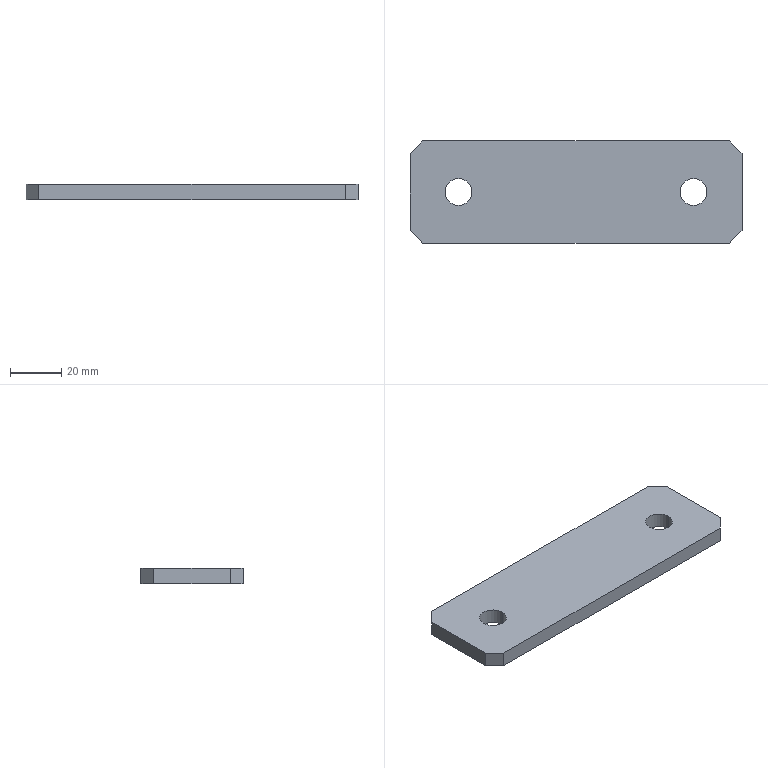Part | SolidWorks | features Extrusion 1 | 1 solid | 14 faces | box 130 x 40 x 6 mm | volume 29861 mm3 | plane 10 | cylinder 4 | commonest cylinder face diameters 10.5 x4
STEP:
#1=CARTESIAN_POINT('',(40.75,0.,3.));
#2=VERTEX_POINT('',#1);
#3=CARTESIAN_POINT('',(51.25,0.,3.));
#4=VERTEX_POINT('',#3);
#5=CARTESIAN_POINT('',(46.,0.,3.));
#6=DIRECTION('',(0.,0.,1.));
#7=DIRECTION('',(1.,0.,0.));
#8=AXIS2_PLACEMENT_3D('',#5,#6,#7);
#9=CIRCLE('',#8,5.25);
#10=EDGE_CURVE('',#2,#4,#9,.T.);
#11=ORIENTED_EDGE('',*,*,#10,.T.);
#12=CARTESIAN_POINT('',(51.25,0.,-3.));
#13=VERTEX_POINT('',#12);
#14=CARTESIAN_POINT('',(51.25,0.,3.));
#15=DIRECTION('',(0.,0.,-1.));
#16=VECTOR('',#15,1000.);
#17=LINE('',#14,#16);
#18=EDGE_CURVE('',#4,#13,#17,.T.);
#19=ORIENTED_EDGE('',*,*,#18,.T.);
#20=CARTESIAN_POINT('',(40.75,0.,-3.));
#21=VERTEX_POINT('',#20);
#22=CARTESIAN_POINT('',(46.,0.,-3.));
#23=DIRECTION('',(0.,0.,1.));
#24=DIRECTION('',(1.,0.,0.));
#25=AXIS2_PLACEMENT_3D('',#22,#23,#24);
#26=CIRCLE('',#25,5.25);
#27=EDGE_CURVE('',#21,#13,#26,.T.);
#28=ORIENTED_EDGE('',*,*,#27,.F.);
#29=CARTESIAN_POINT('',(40.75,0.,3.));
#30=DIRECTION('',(0.,0.,-1.));
#31=VECTOR('',#30,1000.);
#32=LINE('',#29,#31);
#33=EDGE_CURVE('',#2,#21,#32,.T.);
#34=ORIENTED_EDGE('',*,*,#33,.F.);
#35=EDGE_LOOP('',(#11,#19,#28,#34));
#36=FACE_OUTER_BOUND('',#35,.T.);
#37=CARTESIAN_POINT('',(46.,0.,3.));
#38=DIRECTION('',(0.,0.,-1.));
#39=DIRECTION('',(-1.,0.,0.));
#40=AXIS2_PLACEMENT_3D('',#37,#38,#39);
#41=CYLINDRICAL_SURFACE('',#40,5.25);
#42=ADVANCED_FACE('',(#36),#41,.F.);
#43=CARTESIAN_POINT('',(-51.25,0.,3.));
#44=VERTEX_POINT('',#43);
#45=CARTESIAN_POINT('',(-40.75,0.,3.));
#46=VERTEX_POINT('',#45);
#47=CARTESIAN_POINT('',(-46.,0.,3.));
#48=DIRECTION('',(0.,0.,1.));
#49=DIRECTION('',(1.,0.,0.));
#50=AXIS2_PLACEMENT_3D('',#47,#48,#49);
#51=CIRCLE('',#50,5.25);
#52=EDGE_CURVE('',#44,#46,#51,.T.);
#53=ORIENTED_EDGE('',*,*,#52,.T.);
#54=CARTESIAN_POINT('',(-40.75,0.,-3.));
#55=VERTEX_POINT('',#54);
#56=CARTESIAN_POINT('',(-40.75,0.,3.));
#57=DIRECTION('',(0.,0.,-1.));
#58=VECTOR('',#57,1000.);
#59=LINE('',#56,#58);
#60=EDGE_CURVE('',#46,#55,#59,.T.);
#61=ORIENTED_EDGE('',*,*,#60,.T.);
#62=CARTESIAN_POINT('',(-51.25,0.,-3.));
#63=VERTEX_POINT('',#62);
#64=CARTESIAN_POINT('',(-46.,0.,-3.));
#65=DIRECTION('',(0.,0.,1.));
#66=DIRECTION('',(1.,0.,0.));
#67=AXIS2_PLACEMENT_3D('',#64,#65,#66);
#68=CIRCLE('',#67,5.25);
#69=EDGE_CURVE('',#63,#55,#68,.T.);
#70=ORIENTED_EDGE('',*,*,#69,.F.);
#71=CARTESIAN_POINT('',(-51.25,0.,3.));
#72=DIRECTION('',(0.,0.,-1.));
#73=VECTOR('',#72,1000.);
#74=LINE('',#71,#73);
#75=EDGE_CURVE('',#44,#63,#74,.T.);
#76=ORIENTED_EDGE('',*,*,#75,.F.);
#77=EDGE_LOOP('',(#53,#61,#70,#76));
#78=FACE_OUTER_BOUND('',#77,.T.);
#79=CARTESIAN_POINT('',(-46.,0.,3.));
#80=DIRECTION('',(0.,0.,-1.));
#81=DIRECTION('',(-1.,0.,0.));
#82=AXIS2_PLACEMENT_3D('',#79,#80,#81);
#83=CYLINDRICAL_SURFACE('',#82,5.25);
#84=ADVANCED_FACE('',(#78),#83,.F.);
#85=ORIENTED_EDGE('',*,*,#52,.F.);
#86=CARTESIAN_POINT('',(-46.,0.,3.));
#87=DIRECTION('',(0.,0.,1.));
#88=DIRECTION('',(1.,0.,0.));
#89=AXIS2_PLACEMENT_3D('',#86,#87,#88);
#90=CIRCLE('',#89,5.25);
#91=EDGE_CURVE('',#46,#44,#90,.T.);
#92=ORIENTED_EDGE('',*,*,#91,.F.);
#93=EDGE_LOOP('',(#85,#92));
#94=FACE_BOUND('',#93,.T.);
#95=CARTESIAN_POINT('',(-65.,15.,3.));
#96=VERTEX_POINT('',#95);
#97=CARTESIAN_POINT('',(-65.,-15.,3.));
#98=VERTEX_POINT('',#97);
#99=CARTESIAN_POINT('',(-65.,-15.,3.));
#100=DIRECTION('',(0.,-1.,0.));
#101=VECTOR('',#100,1000.);
#102=LINE('',#99,#101);
#103=EDGE_CURVE('',#96,#98,#102,.T.);
#104=ORIENTED_EDGE('',*,*,#103,.T.);
#105=CARTESIAN_POINT('',(-60.,-20.,3.));
#106=VERTEX_POINT('',#105);
#107=CARTESIAN_POINT('',(-60.,-20.,3.));
#108=DIRECTION('',(0.7071,-0.7071,0.));
#109=VECTOR('',#108,1000.);
#110=LINE('',#107,#109);
#111=EDGE_CURVE('',#98,#106,#110,.T.);
#112=ORIENTED_EDGE('',*,*,#111,.T.);
#113=CARTESIAN_POINT('',(60.,-20.,3.));
#114=VERTEX_POINT('',#113);
#115=CARTESIAN_POINT('',(60.,-20.,3.));
#116=DIRECTION('',(1.,0.,0.));
#117=VECTOR('',#116,1000.);
#118=LINE('',#115,#117);
#119=EDGE_CURVE('',#106,#114,#118,.T.);
#120=ORIENTED_EDGE('',*,*,#119,.T.);
#121=CARTESIAN_POINT('',(65.,-15.,3.));
#122=VERTEX_POINT('',#121);
#123=CARTESIAN_POINT('',(65.,-15.,3.));
#124=DIRECTION('',(0.7071,0.7071,0.));
#125=VECTOR('',#124,1000.);
#126=LINE('',#123,#125);
#127=EDGE_CURVE('',#114,#122,#126,.T.);
#128=ORIENTED_EDGE('',*,*,#127,.T.);
#129=CARTESIAN_POINT('',(65.,15.,3.));
#130=VERTEX_POINT('',#129);
#131=CARTESIAN_POINT('',(65.,-15.,3.));
#132=DIRECTION('',(0.,1.,0.));
#133=VECTOR('',#132,1000.);
#134=LINE('',#131,#133);
#135=EDGE_CURVE('',#122,#130,#134,.T.);
#136=ORIENTED_EDGE('',*,*,#135,.T.);
#137=CARTESIAN_POINT('',(60.,20.,3.));
#138=VERTEX_POINT('',#137);
#139=CARTESIAN_POINT('',(65.,15.,3.));
#140=DIRECTION('',(-0.7071,0.7071,0.));
#141=VECTOR('',#140,1000.);
#142=LINE('',#139,#141);
#143=EDGE_CURVE('',#130,#138,#142,.T.);
#144=ORIENTED_EDGE('',*,*,#143,.T.);
#145=CARTESIAN_POINT('',(-60.,20.,3.));
#146=VERTEX_POINT('',#145);
#147=CARTESIAN_POINT('',(60.,20.,3.));
#148=DIRECTION('',(-1.,0.,0.));
#149=VECTOR('',#148,1000.);
#150=LINE('',#147,#149);
#151=EDGE_CURVE('',#138,#146,#150,.T.);
#152=ORIENTED_EDGE('',*,*,#151,.T.);
#153=CARTESIAN_POINT('',(-65.,15.,3.));
#154=DIRECTION('',(-0.7071,-0.7071,0.));
#155=VECTOR('',#154,1000.);
#156=LINE('',#153,#155);
#157=EDGE_CURVE('',#146,#96,#156,.T.);
#158=ORIENTED_EDGE('',*,*,#157,.T.);
#159=EDGE_LOOP('',(#104,#112,#120,#128,#136,#144,#152,#158));
#160=FACE_OUTER_BOUND('',#159,.T.);
#161=ORIENTED_EDGE('',*,*,#10,.F.);
#162=CARTESIAN_POINT('',(46.,0.,3.));
#163=DIRECTION('',(0.,0.,1.));
#164=DIRECTION('',(1.,0.,0.));
#165=AXIS2_PLACEMENT_3D('',#162,#163,#164);
#166=CIRCLE('',#165,5.25);
#167=EDGE_CURVE('',#4,#2,#166,.T.);
#168=ORIENTED_EDGE('',*,*,#167,.F.);
#169=EDGE_LOOP('',(#161,#168));
#170=FACE_BOUND('',#169,.T.);
#171=CARTESIAN_POINT('',(0.,0.,3.));
#172=DIRECTION('',(0.,0.,1.));
#173=DIRECTION('',(1.,0.,0.));
#174=AXIS2_PLACEMENT_3D('',#171,#172,#173);
#175=PLANE('',#174);
#176=ADVANCED_FACE('',(#94,#160,#170),#175,.T.);
#177=CARTESIAN_POINT('',(-65.,15.,-3.));
#178=VERTEX_POINT('',#177);
#179=CARTESIAN_POINT('',(-65.,-15.,-3.));
#180=VERTEX_POINT('',#179);
#181=CARTESIAN_POINT('',(-65.,-15.,-3.));
#182=DIRECTION('',(0.,-1.,0.));
#183=VECTOR('',#182,1000.);
#184=LINE('',#181,#183);
#185=EDGE_CURVE('',#178,#180,#184,.T.);
#186=ORIENTED_EDGE('',*,*,#185,.F.);
#187=CARTESIAN_POINT('',(-60.,20.,-3.));
#188=VERTEX_POINT('',#187);
#189=CARTESIAN_POINT('',(-65.,15.,-3.));
#190=DIRECTION('',(-0.7071,-0.7071,0.));
#191=VECTOR('',#190,1000.);
#192=LINE('',#189,#191);
#193=EDGE_CURVE('',#188,#178,#192,.T.);
#194=ORIENTED_EDGE('',*,*,#193,.F.);
#195=CARTESIAN_POINT('',(60.,20.,-3.));
#196=VERTEX_POINT('',#195);
#197=CARTESIAN_POINT('',(60.,20.,-3.));
#198=DIRECTION('',(-1.,0.,0.));
#199=VECTOR('',#198,1000.);
#200=LINE('',#197,#199);
#201=EDGE_CURVE('',#196,#188,#200,.T.);
#202=ORIENTED_EDGE('',*,*,#201,.F.);
#203=CARTESIAN_POINT('',(65.,15.,-3.));
#204=VERTEX_POINT('',#203);
#205=CARTESIAN_POINT('',(65.,15.,-3.));
#206=DIRECTION('',(-0.7071,0.7071,0.));
#207=VECTOR('',#206,1000.);
#208=LINE('',#205,#207);
#209=EDGE_CURVE('',#204,#196,#208,.T.);
#210=ORIENTED_EDGE('',*,*,#209,.F.);
#211=CARTESIAN_POINT('',(65.,-15.,-3.));
#212=VERTEX_POINT('',#211);
#213=CARTESIAN_POINT('',(65.,-15.,-3.));
#214=DIRECTION('',(0.,1.,0.));
#215=VECTOR('',#214,1000.);
#216=LINE('',#213,#215);
#217=EDGE_CURVE('',#212,#204,#216,.T.);
#218=ORIENTED_EDGE('',*,*,#217,.F.);
#219=CARTESIAN_POINT('',(60.,-20.,-3.));
#220=VERTEX_POINT('',#219);
#221=CARTESIAN_POINT('',(65.,-15.,-3.));
#222=DIRECTION('',(0.7071,0.7071,0.));
#223=VECTOR('',#222,1000.);
#224=LINE('',#221,#223);
#225=EDGE_CURVE('',#220,#212,#224,.T.);
#226=ORIENTED_EDGE('',*,*,#225,.F.);
#227=CARTESIAN_POINT('',(-60.,-20.,-3.));
#228=VERTEX_POINT('',#227);
#229=CARTESIAN_POINT('',(60.,-20.,-3.));
#230=DIRECTION('',(1.,0.,0.));
#231=VECTOR('',#230,1000.);
#232=LINE('',#229,#231);
#233=EDGE_CURVE('',#228,#220,#232,.T.);
#234=ORIENTED_EDGE('',*,*,#233,.F.);
#235=CARTESIAN_POINT('',(-60.,-20.,-3.));
#236=DIRECTION('',(0.7071,-0.7071,0.));
#237=VECTOR('',#236,1000.);
#238=LINE('',#235,#237);
#239=EDGE_CURVE('',#180,#228,#238,.T.);
#240=ORIENTED_EDGE('',*,*,#239,.F.);
#241=EDGE_LOOP('',(#186,#194,#202,#210,#218,#226,#234,#240));
#242=FACE_OUTER_BOUND('',#241,.T.);
#243=ORIENTED_EDGE('',*,*,#69,.T.);
#244=CARTESIAN_POINT('',(-46.,0.,-3.));
#245=DIRECTION('',(0.,0.,1.));
#246=DIRECTION('',(1.,0.,0.));
#247=AXIS2_PLACEMENT_3D('',#244,#245,#246);
#248=CIRCLE('',#247,5.25);
#249=EDGE_CURVE('',#55,#63,#248,.T.);
#250=ORIENTED_EDGE('',*,*,#249,.T.);
#251=EDGE_LOOP('',(#243,#250));
#252=FACE_BOUND('',#251,.T.);
#253=ORIENTED_EDGE('',*,*,#27,.T.);
#254=CARTESIAN_POINT('',(46.,0.,-3.));
#255=DIRECTION('',(0.,0.,1.));
#256=DIRECTION('',(1.,0.,0.));
#257=AXIS2_PLACEMENT_3D('',#254,#255,#256);
#258=CIRCLE('',#257,5.25);
#259=EDGE_CURVE('',#13,#21,#258,.T.);
#260=ORIENTED_EDGE('',*,*,#259,.T.);
#261=EDGE_LOOP('',(#253,#260));
#262=FACE_BOUND('',#261,.T.);
#263=CARTESIAN_POINT('',(0.,0.,-3.));
#264=DIRECTION('',(0.,0.,1.));
#265=DIRECTION('',(1.,0.,0.));
#266=AXIS2_PLACEMENT_3D('',#263,#264,#265);
#267=PLANE('',#266);
#268=ADVANCED_FACE('',(#242,#252,#262),#267,.F.);
#269=ORIENTED_EDGE('',*,*,#185,.T.);
#270=CARTESIAN_POINT('',(-65.,-15.,3.));
#271=DIRECTION('',(0.,0.,-1.));
#272=VECTOR('',#271,1000.);
#273=LINE('',#270,#272);
#274=EDGE_CURVE('',#98,#180,#273,.T.);
#275=ORIENTED_EDGE('',*,*,#274,.F.);
#276=ORIENTED_EDGE('',*,*,#103,.F.);
#277=CARTESIAN_POINT('',(-65.,15.,3.));
#278=DIRECTION('',(0.,0.,-1.));
#279=VECTOR('',#278,1000.);
#280=LINE('',#277,#279);
#281=EDGE_CURVE('',#96,#178,#280,.T.);
#282=ORIENTED_EDGE('',*,*,#281,.T.);
#283=EDGE_LOOP('',(#269,#275,#276,#282));
#284=FACE_OUTER_BOUND('',#283,.T.);
#285=CARTESIAN_POINT('',(-65.,-15.,3.));
#286=DIRECTION('',(1.,0.,0.));
#287=DIRECTION('',(0.,0.,-1.));
#288=AXIS2_PLACEMENT_3D('',#285,#286,#287);
#289=PLANE('',#288);
#290=ADVANCED_FACE('',(#284),#289,.F.);
#291=ORIENTED_EDGE('',*,*,#239,.T.);
#292=CARTESIAN_POINT('',(-60.,-20.,3.));
#293=DIRECTION('',(0.,0.,-1.));
#294=VECTOR('',#293,1000.);
#295=LINE('',#292,#294);
#296=EDGE_CURVE('',#106,#228,#295,.T.);
#297=ORIENTED_EDGE('',*,*,#296,.F.);
#298=ORIENTED_EDGE('',*,*,#111,.F.);
#299=ORIENTED_EDGE('',*,*,#274,.T.);
#300=EDGE_LOOP('',(#291,#297,#298,#299));
#301=FACE_OUTER_BOUND('',#300,.T.);
#302=CARTESIAN_POINT('',(-60.,-20.,3.));
#303=DIRECTION('',(0.7071,0.7071,0.));
#304=DIRECTION('',(-0.7071,0.7071,0.));
#305=AXIS2_PLACEMENT_3D('',#302,#303,#304);
#306=PLANE('',#305);
#307=ADVANCED_FACE('',(#301),#306,.F.);
#308=ORIENTED_EDGE('',*,*,#233,.T.);
#309=CARTESIAN_POINT('',(60.,-20.,3.));
#310=DIRECTION('',(0.,0.,-1.));
#311=VECTOR('',#310,1000.);
#312=LINE('',#309,#311);
#313=EDGE_CURVE('',#114,#220,#312,.T.);
#314=ORIENTED_EDGE('',*,*,#313,.F.);
#315=ORIENTED_EDGE('',*,*,#119,.F.);
#316=ORIENTED_EDGE('',*,*,#296,.T.);
#317=EDGE_LOOP('',(#308,#314,#315,#316));
#318=FACE_OUTER_BOUND('',#317,.T.);
#319=CARTESIAN_POINT('',(60.,-20.,3.));
#320=DIRECTION('',(0.,1.,0.));
#321=DIRECTION('',(-1.,0.,0.));
#322=AXIS2_PLACEMENT_3D('',#319,#320,#321);
#323=PLANE('',#322);
#324=ADVANCED_FACE('',(#318),#323,.F.);
#325=ORIENTED_EDGE('',*,*,#225,.T.);
#326=CARTESIAN_POINT('',(65.,-15.,3.));
#327=DIRECTION('',(0.,0.,-1.));
#328=VECTOR('',#327,1000.);
#329=LINE('',#326,#328);
#330=EDGE_CURVE('',#122,#212,#329,.T.);
#331=ORIENTED_EDGE('',*,*,#330,.F.);
#332=ORIENTED_EDGE('',*,*,#127,.F.);
#333=ORIENTED_EDGE('',*,*,#313,.T.);
#334=EDGE_LOOP('',(#325,#331,#332,#333));
#335=FACE_OUTER_BOUND('',#334,.T.);
#336=CARTESIAN_POINT('',(65.,-15.,3.));
#337=DIRECTION('',(-0.7071,0.7071,0.));
#338=DIRECTION('',(-0.7071,-0.7071,0.));
#339=AXIS2_PLACEMENT_3D('',#336,#337,#338);
#340=PLANE('',#339);
#341=ADVANCED_FACE('',(#335),#340,.F.);
#342=ORIENTED_EDGE('',*,*,#217,.T.);
#343=CARTESIAN_POINT('',(65.,15.,3.));
#344=DIRECTION('',(0.,0.,-1.));
#345=VECTOR('',#344,1000.);
#346=LINE('',#343,#345);
#347=EDGE_CURVE('',#130,#204,#346,.T.);
#348=ORIENTED_EDGE('',*,*,#347,.F.);
#349=ORIENTED_EDGE('',*,*,#135,.F.);
#350=ORIENTED_EDGE('',*,*,#330,.T.);
#351=EDGE_LOOP('',(#342,#348,#349,#350));
#352=FACE_OUTER_BOUND('',#351,.T.);
#353=CARTESIAN_POINT('',(65.,-15.,3.));
#354=DIRECTION('',(-1.,0.,0.));
#355=DIRECTION('',(0.,0.,1.));
#356=AXIS2_PLACEMENT_3D('',#353,#354,#355);
#357=PLANE('',#356);
#358=ADVANCED_FACE('',(#352),#357,.F.);
#359=ORIENTED_EDGE('',*,*,#209,.T.);
#360=CARTESIAN_POINT('',(60.,20.,3.));
#361=DIRECTION('',(0.,0.,-1.));
#362=VECTOR('',#361,1000.);
#363=LINE('',#360,#362);
#364=EDGE_CURVE('',#138,#196,#363,.T.);
#365=ORIENTED_EDGE('',*,*,#364,.F.);
#366=ORIENTED_EDGE('',*,*,#143,.F.);
#367=ORIENTED_EDGE('',*,*,#347,.T.);
#368=EDGE_LOOP('',(#359,#365,#366,#367));
#369=FACE_OUTER_BOUND('',#368,.T.);
#370=CARTESIAN_POINT('',(65.,15.,3.));
#371=DIRECTION('',(-0.7071,-0.7071,0.));
#372=DIRECTION('',(0.7071,-0.7071,0.));
#373=AXIS2_PLACEMENT_3D('',#370,#371,#372);
#374=PLANE('',#373);
#375=ADVANCED_FACE('',(#369),#374,.F.);
#376=ORIENTED_EDGE('',*,*,#201,.T.);
#377=CARTESIAN_POINT('',(-60.,20.,3.));
#378=DIRECTION('',(0.,0.,-1.));
#379=VECTOR('',#378,1000.);
#380=LINE('',#377,#379);
#381=EDGE_CURVE('',#146,#188,#380,.T.);
#382=ORIENTED_EDGE('',*,*,#381,.F.);
#383=ORIENTED_EDGE('',*,*,#151,.F.);
#384=ORIENTED_EDGE('',*,*,#364,.T.);
#385=EDGE_LOOP('',(#376,#382,#383,#384));
#386=FACE_OUTER_BOUND('',#385,.T.);
#387=CARTESIAN_POINT('',(60.,20.,3.));
#388=DIRECTION('',(0.,-1.,0.));
#389=DIRECTION('',(1.,0.,0.));
#390=AXIS2_PLACEMENT_3D('',#387,#388,#389);
#391=PLANE('',#390);
#392=ADVANCED_FACE('',(#386),#391,.F.);
#393=ORIENTED_EDGE('',*,*,#193,.T.);
#394=ORIENTED_EDGE('',*,*,#281,.F.);
#395=ORIENTED_EDGE('',*,*,#157,.F.);
#396=ORIENTED_EDGE('',*,*,#381,.T.);
#397=EDGE_LOOP('',(#393,#394,#395,#396));
#398=FACE_OUTER_BOUND('',#397,.T.);
#399=CARTESIAN_POINT('',(-65.,15.,3.));
#400=DIRECTION('',(0.7071,-0.7071,0.));
#401=DIRECTION('',(0.7071,0.7071,0.));
#402=AXIS2_PLACEMENT_3D('',#399,#400,#401);
#403=PLANE('',#402);
#404=ADVANCED_FACE('',(#398),#403,.F.);
#405=ORIENTED_EDGE('',*,*,#60,.F.);
#406=ORIENTED_EDGE('',*,*,#91,.T.);
#407=ORIENTED_EDGE('',*,*,#75,.T.);
#408=ORIENTED_EDGE('',*,*,#249,.F.);
#409=EDGE_LOOP('',(#405,#406,#407,#408));
#410=FACE_OUTER_BOUND('',#409,.T.);
#411=CARTESIAN_POINT('',(-46.,0.,3.));
#412=DIRECTION('',(0.,0.,-1.));
#413=DIRECTION('',(-1.,0.,0.));
#414=AXIS2_PLACEMENT_3D('',#411,#412,#413);
#415=CYLINDRICAL_SURFACE('',#414,5.25);
#416=ADVANCED_FACE('',(#410),#415,.F.);
#417=ORIENTED_EDGE('',*,*,#18,.F.);
#418=ORIENTED_EDGE('',*,*,#167,.T.);
#419=ORIENTED_EDGE('',*,*,#33,.T.);
#420=ORIENTED_EDGE('',*,*,#259,.F.);
#421=EDGE_LOOP('',(#417,#418,#419,#420));
#422=FACE_OUTER_BOUND('',#421,.T.);
#423=CARTESIAN_POINT('',(46.,0.,3.));
#424=DIRECTION('',(0.,0.,-1.));
#425=DIRECTION('',(-1.,0.,0.));
#426=AXIS2_PLACEMENT_3D('',#423,#424,#425);
#427=CYLINDRICAL_SURFACE('',#426,5.25);
#428=ADVANCED_FACE('',(#422),#427,.F.);
#429=CLOSED_SHELL('',(#42,#84,#176,#268,#290,#307,#324,#341,#358,#375,#392,#404,#416,#428));
#430=MANIFOLD_SOLID_BREP('',#429);
#431=CARTESIAN_POINT('',(0.,0.,0.));
#432=DIRECTION('',(0.,0.,1.));
#433=DIRECTION('',(1.,0.,0.));
#434=AXIS2_PLACEMENT_3D('',#431,#432,#433);
#435=(LENGTH_UNIT()NAMED_UNIT(*)SI_UNIT(.MILLI.,.METRE.));
#436=UNCERTAINTY_MEASURE_WITH_UNIT(LENGTH_MEASURE(0.00001),#435,'','');
#437=(NAMED_UNIT(*)PLANE_ANGLE_UNIT()SI_UNIT($,.RADIAN.));
#438=(NAMED_UNIT(*)SI_UNIT($,.STERADIAN.)SOLID_ANGLE_UNIT());
#439=(GEOMETRIC_REPRESENTATION_CONTEXT(3)GLOBAL_UNCERTAINTY_ASSIGNED_CONTEXT((#436))GLOBAL_UNIT_ASSIGNED_CONTEXT((#435,#437,#438))REPRESENTATION_CONTEXT('',''));
#440=ADVANCED_BREP_SHAPE_REPRESENTATION('',(#430,#434),#439);